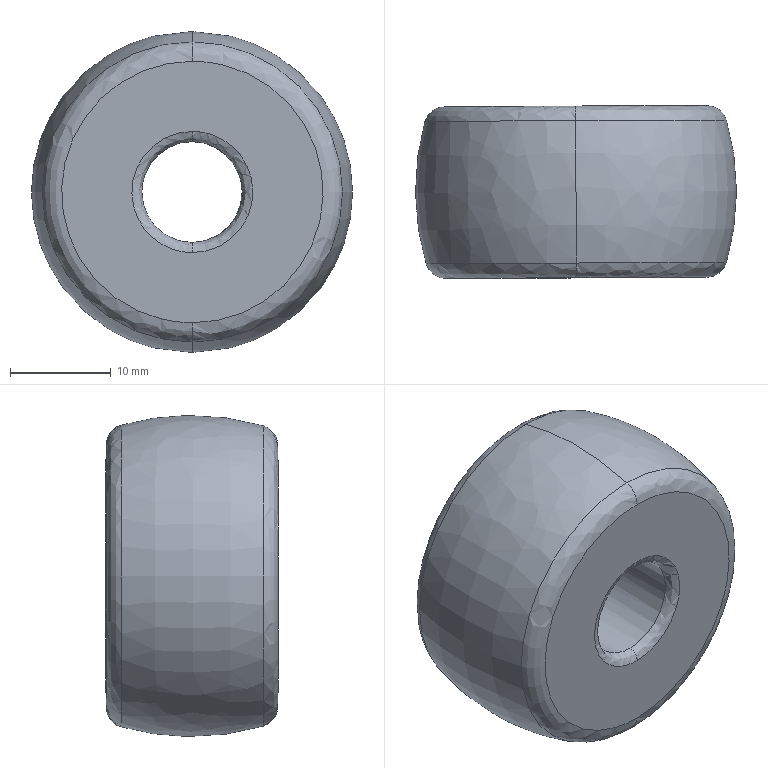Part | SolidWorks | features BaseBody 1 | 1 solid | 14 faces | box 31.826 x 17.113 x 31.826 mm | volume 11303 mm3 | spline 10 | cylinder 2 | plane 2 | commonest cylinder face diameters 10 x2
STEP:
#1=CARTESIAN_POINT('',(616.883,-156.463,-67.113));
#2=VERTEX_POINT('',#1);
#3=CARTESIAN_POINT('',(616.883,-156.463,-37.355));
#4=VERTEX_POINT('',#3);
#5=CARTESIAN_POINT('',(616.883,-156.463,-52.234));
#6=DIRECTION('',(0.004352,-1.,-0.000000003));
#7=DIRECTION('',(0.000000001,-0.000000003,1.));
#8=AXIS2_PLACEMENT_3D('',#5,#6,#7);
#9=CIRCLE('',#8,14.879);
#10=EDGE_CURVE('',#2,#4,#9,.T.);
#11=ORIENTED_EDGE('',*,*,#10,.F.);
#12=CARTESIAN_POINT('',(616.822,-142.349,-67.176));
#13=VERTEX_POINT('',#12);
#14=CARTESIAN_POINT('',(616.883,-156.463,-67.113));
#15=CARTESIAN_POINT('',(616.878,-155.365,-67.437));
#16=CARTESIAN_POINT('',(616.868,-153.033,-67.956));
#17=CARTESIAN_POINT('',(616.852,-149.411,-68.238));
#18=CARTESIAN_POINT('',(616.837,-145.786,-67.988));
#19=CARTESIAN_POINT('',(616.826,-143.45,-67.49));
#20=CARTESIAN_POINT('',(616.822,-142.349,-67.176));
#21=B_SPLINE_CURVE_WITH_KNOTS('',3,(#14,#15,#16,#17,#18,#19,#20),.UNSPECIFIED.,.F.,.F.,(4,1,1,1,4),(0.01923,0.25,0.5,0.75,0.9808),.UNSPECIFIED.);
#22=EDGE_CURVE('',#2,#13,#21,.T.);
#23=ORIENTED_EDGE('',*,*,#22,.T.);
#24=CARTESIAN_POINT('',(616.822,-142.349,-37.292));
#25=VERTEX_POINT('',#24);
#26=CARTESIAN_POINT('',(616.822,-142.349,-52.234));
#27=DIRECTION('',(-0.004352,1.,0.000000003));
#28=DIRECTION('',(0.000000001,-0.000000003,1.));
#29=AXIS2_PLACEMENT_3D('',#26,#27,#28);
#30=CIRCLE('',#29,14.942);
#31=EDGE_CURVE('',#25,#13,#30,.T.);
#32=ORIENTED_EDGE('',*,*,#31,.F.);
#33=CARTESIAN_POINT('',(616.883,-156.463,-37.355));
#34=CARTESIAN_POINT('',(616.878,-155.365,-37.031));
#35=CARTESIAN_POINT('',(616.868,-153.033,-36.513));
#36=CARTESIAN_POINT('',(616.852,-149.411,-36.23));
#37=CARTESIAN_POINT('',(616.837,-145.786,-36.48));
#38=CARTESIAN_POINT('',(616.826,-143.45,-36.979));
#39=CARTESIAN_POINT('',(616.822,-142.349,-37.292));
#40=B_SPLINE_CURVE_WITH_KNOTS('',3,(#33,#34,#35,#36,#37,#38,#39),.UNSPECIFIED.,.F.,.F.,(4,1,1,1,4),(0.01923,0.25,0.5,0.75,0.9808),.UNSPECIFIED.);
#41=EDGE_CURVE('',#4,#25,#40,.T.);
#42=ORIENTED_EDGE('',*,*,#41,.F.);
#43=EDGE_LOOP('',(#11,#23,#32,#42));
#44=FACE_OUTER_BOUND('',#43,.T.);
#45=CARTESIAN_POINT('',(616.883,-156.463,-37.355));
#46=CARTESIAN_POINT('',(646.641,-156.333,-37.355));
#47=CARTESIAN_POINT('',(646.641,-156.333,-67.113));
#48=CARTESIAN_POINT('',(616.883,-156.463,-67.113));
#49=CARTESIAN_POINT('',(616.878,-155.365,-37.031));
#50=CARTESIAN_POINT('',(647.284,-155.233,-37.031));
#51=CARTESIAN_POINT('',(647.284,-155.233,-67.437));
#52=CARTESIAN_POINT('',(616.878,-155.365,-67.437));
#53=CARTESIAN_POINT('',(616.868,-153.033,-36.513));
#54=CARTESIAN_POINT('',(648.311,-152.896,-36.513));
#55=CARTESIAN_POINT('',(648.311,-152.896,-67.956));
#56=CARTESIAN_POINT('',(616.868,-153.033,-67.956));
#57=CARTESIAN_POINT('',(616.852,-149.411,-36.23));
#58=CARTESIAN_POINT('',(648.86,-149.272,-36.23));
#59=CARTESIAN_POINT('',(648.86,-149.272,-68.238));
#60=CARTESIAN_POINT('',(616.852,-149.411,-68.238));
#61=CARTESIAN_POINT('',(616.837,-145.786,-36.48));
#62=CARTESIAN_POINT('',(648.344,-145.649,-36.48));
#63=CARTESIAN_POINT('',(648.344,-145.649,-67.988));
#64=CARTESIAN_POINT('',(616.837,-145.786,-67.988));
#65=CARTESIAN_POINT('',(616.826,-143.45,-36.979));
#66=CARTESIAN_POINT('',(647.337,-143.317,-36.979));
#67=CARTESIAN_POINT('',(647.337,-143.317,-67.49));
#68=CARTESIAN_POINT('',(616.826,-143.45,-67.49));
#69=CARTESIAN_POINT('',(616.822,-142.349,-37.292));
#70=CARTESIAN_POINT('',(646.705,-142.219,-37.292));
#71=CARTESIAN_POINT('',(646.705,-142.219,-67.176));
#72=CARTESIAN_POINT('',(616.822,-142.349,-67.176));
#73=(BOUNDED_SURFACE()B_SPLINE_SURFACE(3,3,((#45,#46,#47,#48),(#49,#50,#51,#52),(#53,#54,#55,#56),(#57,#58,#59,#60),(#61,#62,#63,#64),(#65,#66,#67,#68),(#69,#70,#71,#72)),.UNSPECIFIED.,.F.,.F.,.F.)B_SPLINE_SURFACE_WITH_KNOTS((4,1,1,1,4),(4,4),(0.01923,0.25,0.5,0.75,0.9808),(0.,1.),.UNSPECIFIED.)GEOMETRIC_REPRESENTATION_ITEM()RATIONAL_B_SPLINE_SURFACE(((1.,0.3333,0.3333,1.),(1.,0.3333,0.3333,1.),(1.,0.3333,0.3333,1.),(1.,0.3333,0.3333,1.),(1.,0.3333,0.3333,1.),(1.,0.3333,0.3333,1.),(1.,0.3333,0.3333,1.)))REPRESENTATION_ITEM('')SURFACE());
#74=ADVANCED_FACE('',(#44),#73,.F.);
#75=ORIENTED_EDGE('',*,*,#31,.T.);
#76=CARTESIAN_POINT('',(616.815,-140.898,-65.253));
#77=VERTEX_POINT('',#76);
#78=CARTESIAN_POINT('',(616.822,-142.349,-67.176));
#79=CARTESIAN_POINT('',(616.821,-142.15,-67.119));
#80=CARTESIAN_POINT('',(616.819,-141.754,-66.936));
#81=CARTESIAN_POINT('',(616.817,-141.271,-66.48));
#82=CARTESIAN_POINT('',(616.816,-140.965,-65.89));
#83=CARTESIAN_POINT('',(616.815,-140.898,-65.459));
#84=CARTESIAN_POINT('',(616.815,-140.898,-65.253));
#85=B_SPLINE_CURVE_WITH_KNOTS('',3,(#78,#79,#80,#81,#82,#83,#84),.UNSPECIFIED.,.F.,.F.,(4,1,1,1,4),(0.01923,0.25,0.5,0.75,0.9808),.UNSPECIFIED.);
#86=EDGE_CURVE('',#13,#77,#85,.T.);
#87=ORIENTED_EDGE('',*,*,#86,.T.);
#88=CARTESIAN_POINT('',(616.815,-140.898,-39.216));
#89=VERTEX_POINT('',#88);
#90=CARTESIAN_POINT('',(616.815,-140.898,-39.216));
#91=CARTESIAN_POINT('',(617.67,-140.894,-39.216));
#92=CARTESIAN_POINT('',(618.517,-140.89,-39.299));
#93=CARTESIAN_POINT('',(620.193,-140.883,-39.632));
#94=CARTESIAN_POINT('',(621.008,-140.879,-39.88));
#95=CARTESIAN_POINT('',(622.587,-140.872,-40.534));
#96=CARTESIAN_POINT('',(623.338,-140.869,-40.935));
#97=CARTESIAN_POINT('',(624.758,-140.863,-41.884));
#98=CARTESIAN_POINT('',(625.417,-140.86,-42.425));
#99=CARTESIAN_POINT('',(626.625,-140.855,-43.633));
#100=CARTESIAN_POINT('',(627.165,-140.853,-44.291));
#101=CARTESIAN_POINT('',(628.114,-140.848,-45.712));
#102=CARTESIAN_POINT('',(628.516,-140.847,-46.463));
#103=CARTESIAN_POINT('',(629.17,-140.844,-48.042));
#104=CARTESIAN_POINT('',(629.417,-140.843,-48.856));
#105=CARTESIAN_POINT('',(629.75,-140.841,-50.532));
#106=CARTESIAN_POINT('',(629.834,-140.841,-51.38));
#107=CARTESIAN_POINT('',(629.834,-140.841,-53.089));
#108=CARTESIAN_POINT('',(629.75,-140.841,-53.936));
#109=CARTESIAN_POINT('',(629.417,-140.843,-55.612));
#110=CARTESIAN_POINT('',(629.17,-140.844,-56.427));
#111=CARTESIAN_POINT('',(628.516,-140.847,-58.005));
#112=CARTESIAN_POINT('',(628.114,-140.848,-58.756));
#113=CARTESIAN_POINT('',(627.165,-140.853,-60.177));
#114=CARTESIAN_POINT('',(626.625,-140.855,-60.835));
#115=CARTESIAN_POINT('',(625.417,-140.86,-62.044));
#116=CARTESIAN_POINT('',(624.758,-140.863,-62.584));
#117=CARTESIAN_POINT('',(623.338,-140.869,-63.533));
#118=CARTESIAN_POINT('',(622.587,-140.872,-63.935));
#119=CARTESIAN_POINT('',(621.008,-140.879,-64.589));
#120=CARTESIAN_POINT('',(620.193,-140.883,-64.836));
#121=CARTESIAN_POINT('',(618.517,-140.89,-65.169));
#122=CARTESIAN_POINT('',(617.67,-140.894,-65.253));
#123=CARTESIAN_POINT('',(616.815,-140.898,-65.253));
#124=B_SPLINE_CURVE_WITH_KNOTS('',3,(#90,#91,#92,#93,#94,#95,#96,#97,#98,#99,#100,#101,#102,#103,#104,#105,#106,#107,#108,#109,#110,#111,#112,#113,#114,#115,#116,#117,#118,#119,#120,#121,#122,#123),.UNSPECIFIED.,.F.,.F.,(4,2,2,2,2,2,2,2,2,2,2,2,2,2,2,2,4),(0.,0.0625,0.125,0.1875,0.25,0.3125,0.375,0.4375,0.5,0.5625,0.625,0.6875,0.75,0.8125,0.875,0.9375,1.),.UNSPECIFIED.);
#125=EDGE_CURVE('',#89,#77,#124,.T.);
#126=ORIENTED_EDGE('',*,*,#125,.F.);
#127=CARTESIAN_POINT('',(616.822,-142.349,-37.292));
#128=CARTESIAN_POINT('',(616.821,-142.15,-37.349));
#129=CARTESIAN_POINT('',(616.819,-141.754,-37.532));
#130=CARTESIAN_POINT('',(616.817,-141.271,-37.988));
#131=CARTESIAN_POINT('',(616.816,-140.965,-38.578));
#132=CARTESIAN_POINT('',(616.815,-140.898,-39.009));
#133=CARTESIAN_POINT('',(616.815,-140.898,-39.216));
#134=B_SPLINE_CURVE_WITH_KNOTS('',3,(#127,#128,#129,#130,#131,#132,#133),.UNSPECIFIED.,.F.,.F.,(4,1,1,1,4),(0.01923,0.25,0.5,0.75,0.9808),.UNSPECIFIED.);
#135=EDGE_CURVE('',#25,#89,#134,.T.);
#136=ORIENTED_EDGE('',*,*,#135,.F.);
#137=EDGE_LOOP('',(#75,#87,#126,#136));
#138=FACE_OUTER_BOUND('',#137,.T.);
#139=CARTESIAN_POINT('',(616.822,-142.349,-37.292));
#140=CARTESIAN_POINT('',(646.705,-142.219,-37.292));
#141=CARTESIAN_POINT('',(646.705,-142.219,-67.176));
#142=CARTESIAN_POINT('',(616.822,-142.349,-67.176));
#143=CARTESIAN_POINT('',(616.821,-142.15,-37.349));
#144=CARTESIAN_POINT('',(646.591,-142.021,-37.349));
#145=CARTESIAN_POINT('',(646.591,-142.021,-67.119));
#146=CARTESIAN_POINT('',(616.821,-142.15,-67.119));
#147=CARTESIAN_POINT('',(616.819,-141.754,-37.532));
#148=CARTESIAN_POINT('',(646.223,-141.626,-37.532));
#149=CARTESIAN_POINT('',(646.223,-141.626,-66.936));
#150=CARTESIAN_POINT('',(616.819,-141.754,-66.936));
#151=CARTESIAN_POINT('',(616.817,-141.271,-37.988));
#152=CARTESIAN_POINT('',(645.309,-141.147,-37.988));
#153=CARTESIAN_POINT('',(645.309,-141.147,-66.48));
#154=CARTESIAN_POINT('',(616.817,-141.271,-66.48));
#155=CARTESIAN_POINT('',(616.816,-140.965,-38.578));
#156=CARTESIAN_POINT('',(644.128,-140.846,-38.578));
#157=CARTESIAN_POINT('',(644.128,-140.846,-65.89));
#158=CARTESIAN_POINT('',(616.816,-140.965,-65.89));
#159=CARTESIAN_POINT('',(616.815,-140.898,-39.009));
#160=CARTESIAN_POINT('',(643.266,-140.782,-39.009));
#161=CARTESIAN_POINT('',(643.266,-140.782,-65.459));
#162=CARTESIAN_POINT('',(616.815,-140.898,-65.459));
#163=CARTESIAN_POINT('',(616.815,-140.898,-39.216));
#164=CARTESIAN_POINT('',(642.852,-140.784,-39.216));
#165=CARTESIAN_POINT('',(642.852,-140.784,-65.253));
#166=CARTESIAN_POINT('',(616.815,-140.898,-65.253));
#167=(BOUNDED_SURFACE()B_SPLINE_SURFACE(3,3,((#139,#140,#141,#142),(#143,#144,#145,#146),(#147,#148,#149,#150),(#151,#152,#153,#154),(#155,#156,#157,#158),(#159,#160,#161,#162),(#163,#164,#165,#166)),.UNSPECIFIED.,.F.,.F.,.F.)B_SPLINE_SURFACE_WITH_KNOTS((4,1,1,1,4),(4,4),(0.01923,0.25,0.5,0.75,0.9808),(0.,1.),.UNSPECIFIED.)GEOMETRIC_REPRESENTATION_ITEM()RATIONAL_B_SPLINE_SURFACE(((1.,0.3333,0.3333,1.),(1.,0.3333,0.3333,1.),(1.,0.3333,0.3333,1.),(1.,0.3333,0.3333,1.),(1.,0.3333,0.3333,1.),(1.,0.3333,0.3333,1.),(1.,0.3333,0.3333,1.)))REPRESENTATION_ITEM('')SURFACE());
#168=ADVANCED_FACE('',(#138),#167,.F.);
#169=CARTESIAN_POINT('',(616.889,-157.897,-65.195));
#170=VERTEX_POINT('',#169);
#171=CARTESIAN_POINT('',(616.889,-157.897,-39.273));
#172=VERTEX_POINT('',#171);
#173=CARTESIAN_POINT('',(616.889,-157.897,-65.195));
#174=CARTESIAN_POINT('',(617.74,-157.894,-65.195));
#175=CARTESIAN_POINT('',(618.584,-157.89,-65.112));
#176=CARTESIAN_POINT('',(620.252,-157.883,-64.78));
#177=CARTESIAN_POINT('',(621.063,-157.879,-64.534));
#178=CARTESIAN_POINT('',(622.635,-157.872,-63.883));
#179=CARTESIAN_POINT('',(623.383,-157.869,-63.483));
#180=CARTESIAN_POINT('',(624.797,-157.863,-62.538));
#181=CARTESIAN_POINT('',(625.452,-157.86,-62.));
#182=CARTESIAN_POINT('',(626.656,-157.855,-60.797));
#183=CARTESIAN_POINT('',(627.193,-157.853,-60.142));
#184=CARTESIAN_POINT('',(628.138,-157.848,-58.728));
#185=CARTESIAN_POINT('',(628.538,-157.847,-57.98));
#186=CARTESIAN_POINT('',(629.189,-157.844,-56.408));
#187=CARTESIAN_POINT('',(629.435,-157.843,-55.597));
#188=CARTESIAN_POINT('',(629.767,-157.841,-53.928));
#189=CARTESIAN_POINT('',(629.85,-157.841,-53.085));
#190=CARTESIAN_POINT('',(629.85,-157.841,-51.383));
#191=CARTESIAN_POINT('',(629.767,-157.841,-50.54));
#192=CARTESIAN_POINT('',(629.435,-157.843,-48.871));
#193=CARTESIAN_POINT('',(629.189,-157.844,-48.06));
#194=CARTESIAN_POINT('',(628.538,-157.847,-46.488));
#195=CARTESIAN_POINT('',(628.138,-157.848,-45.741));
#196=CARTESIAN_POINT('',(627.193,-157.853,-44.326));
#197=CARTESIAN_POINT('',(626.655,-157.855,-43.671));
#198=CARTESIAN_POINT('',(625.453,-157.86,-42.468));
#199=CARTESIAN_POINT('',(624.797,-157.863,-41.93));
#200=CARTESIAN_POINT('',(623.383,-157.869,-40.985));
#201=CARTESIAN_POINT('',(622.635,-157.872,-40.585));
#202=CARTESIAN_POINT('',(621.063,-157.879,-39.934));
#203=CARTESIAN_POINT('',(620.252,-157.883,-39.688));
#204=CARTESIAN_POINT('',(618.583,-157.89,-39.356));
#205=CARTESIAN_POINT('',(617.741,-157.894,-39.273));
#206=CARTESIAN_POINT('',(616.889,-157.897,-39.273));
#207=B_SPLINE_CURVE_WITH_KNOTS('',3,(#173,#174,#175,#176,#177,#178,#179,#180,#181,#182,#183,#184,#185,#186,#187,#188,#189,#190,#191,#192,#193,#194,#195,#196,#197,#198,#199,#200,#201,#202,#203,#204,#205,#206),.UNSPECIFIED.,.F.,.F.,(4,2,2,2,2,2,2,2,2,2,2,2,2,2,2,2,4),(0.,0.0625,0.125,0.1875,0.25,0.3125,0.375,0.4375,0.5,0.5625,0.625,0.6875,0.75,0.8125,0.875,0.9375,1.),.UNSPECIFIED.);
#208=EDGE_CURVE('',#170,#172,#207,.T.);
#209=ORIENTED_EDGE('',*,*,#208,.F.);
#210=CARTESIAN_POINT('',(616.889,-157.897,-65.195));
#211=CARTESIAN_POINT('',(616.889,-157.897,-65.4));
#212=CARTESIAN_POINT('',(616.889,-157.831,-65.829));
#213=CARTESIAN_POINT('',(616.888,-157.529,-66.415));
#214=CARTESIAN_POINT('',(616.886,-157.052,-66.871));
#215=CARTESIAN_POINT('',(616.884,-156.66,-67.055));
#216=CARTESIAN_POINT('',(616.883,-156.463,-67.113));
#217=B_SPLINE_CURVE_WITH_KNOTS('',3,(#210,#211,#212,#213,#214,#215,#216),.UNSPECIFIED.,.F.,.F.,(4,1,1,1,4),(0.01923,0.25,0.5,0.75,0.9808),.UNSPECIFIED.);
#218=EDGE_CURVE('',#170,#2,#217,.T.);
#219=ORIENTED_EDGE('',*,*,#218,.T.);
#220=ORIENTED_EDGE('',*,*,#10,.T.);
#221=CARTESIAN_POINT('',(616.889,-157.897,-39.273));
#222=CARTESIAN_POINT('',(616.889,-157.897,-39.068));
#223=CARTESIAN_POINT('',(616.889,-157.831,-38.64));
#224=CARTESIAN_POINT('',(616.888,-157.529,-38.053));
#225=CARTESIAN_POINT('',(616.886,-157.052,-37.598));
#226=CARTESIAN_POINT('',(616.884,-156.66,-37.413));
#227=CARTESIAN_POINT('',(616.883,-156.463,-37.355));
#228=B_SPLINE_CURVE_WITH_KNOTS('',3,(#221,#222,#223,#224,#225,#226,#227),.UNSPECIFIED.,.F.,.F.,(4,1,1,1,4),(0.01923,0.25,0.5,0.75,0.9808),.UNSPECIFIED.);
#229=EDGE_CURVE('',#172,#4,#228,.T.);
#230=ORIENTED_EDGE('',*,*,#229,.F.);
#231=EDGE_LOOP('',(#209,#219,#220,#230));
#232=FACE_OUTER_BOUND('',#231,.T.);
#233=CARTESIAN_POINT('',(616.889,-157.897,-39.273));
#234=CARTESIAN_POINT('',(642.811,-157.785,-39.273));
#235=CARTESIAN_POINT('',(642.811,-157.785,-65.195));
#236=CARTESIAN_POINT('',(616.889,-157.897,-65.195));
#237=CARTESIAN_POINT('',(616.889,-157.897,-39.068));
#238=CARTESIAN_POINT('',(643.222,-157.783,-39.068));
#239=CARTESIAN_POINT('',(643.222,-157.783,-65.4));
#240=CARTESIAN_POINT('',(616.889,-157.897,-65.4));
#241=CARTESIAN_POINT('',(616.889,-157.831,-38.64));
#242=CARTESIAN_POINT('',(644.078,-157.713,-38.64));
#243=CARTESIAN_POINT('',(644.078,-157.713,-65.829));
#244=CARTESIAN_POINT('',(616.889,-157.831,-65.829));
#245=CARTESIAN_POINT('',(616.888,-157.529,-38.053));
#246=CARTESIAN_POINT('',(645.25,-157.406,-38.053));
#247=CARTESIAN_POINT('',(645.25,-157.406,-66.415));
#248=CARTESIAN_POINT('',(616.888,-157.529,-66.415));
#249=CARTESIAN_POINT('',(616.886,-157.052,-37.598));
#250=CARTESIAN_POINT('',(646.158,-156.924,-37.598));
#251=CARTESIAN_POINT('',(646.158,-156.924,-66.871));
#252=CARTESIAN_POINT('',(616.886,-157.052,-66.871));
#253=CARTESIAN_POINT('',(616.884,-156.66,-37.413));
#254=CARTESIAN_POINT('',(646.526,-156.531,-37.413));
#255=CARTESIAN_POINT('',(646.526,-156.531,-67.055));
#256=CARTESIAN_POINT('',(616.884,-156.66,-67.055));
#257=CARTESIAN_POINT('',(616.883,-156.463,-37.355));
#258=CARTESIAN_POINT('',(646.641,-156.333,-37.355));
#259=CARTESIAN_POINT('',(646.641,-156.333,-67.113));
#260=CARTESIAN_POINT('',(616.883,-156.463,-67.113));
#261=(BOUNDED_SURFACE()B_SPLINE_SURFACE(3,3,((#233,#234,#235,#236),(#237,#238,#239,#240),(#241,#242,#243,#244),(#245,#246,#247,#248),(#249,#250,#251,#252),(#253,#254,#255,#256),(#257,#258,#259,#260)),.UNSPECIFIED.,.F.,.F.,.F.)B_SPLINE_SURFACE_WITH_KNOTS((4,1,1,1,4),(4,4),(0.01923,0.25,0.5,0.75,0.9808),(0.,1.),.UNSPECIFIED.)GEOMETRIC_REPRESENTATION_ITEM()RATIONAL_B_SPLINE_SURFACE(((1.,0.3333,0.3333,1.),(1.,0.3333,0.3333,1.),(1.,0.3333,0.3333,1.),(1.,0.3333,0.3333,1.),(1.,0.3333,0.3333,1.),(1.,0.3333,0.3333,1.),(1.,0.3333,0.3333,1.)))REPRESENTATION_ITEM('')SURFACE());
#262=ADVANCED_FACE('',(#232),#261,.F.);
#263=CARTESIAN_POINT('',(616.815,-140.898,-58.234));
#264=VERTEX_POINT('',#263);
#265=CARTESIAN_POINT('',(616.815,-140.898,-46.234));
#266=VERTEX_POINT('',#265);
#267=CARTESIAN_POINT('',(616.815,-140.898,-58.234));
#268=CARTESIAN_POINT('',(617.603,-140.894,-58.234));
#269=CARTESIAN_POINT('',(618.384,-140.891,-58.079));
#270=CARTESIAN_POINT('',(619.839,-140.884,-57.476));
#271=CARTESIAN_POINT('',(620.501,-140.882,-57.033));
#272=CARTESIAN_POINT('',(621.615,-140.877,-55.92));
#273=CARTESIAN_POINT('',(622.057,-140.875,-55.257));
#274=CARTESIAN_POINT('',(622.66,-140.872,-53.803));
#275=CARTESIAN_POINT('',(622.815,-140.871,-53.021));
#276=CARTESIAN_POINT('',(622.815,-140.871,-51.447));
#277=CARTESIAN_POINT('',(622.66,-140.872,-50.665));
#278=CARTESIAN_POINT('',(622.057,-140.875,-49.211));
#279=CARTESIAN_POINT('',(621.615,-140.877,-48.548));
#280=CARTESIAN_POINT('',(620.501,-140.882,-47.435));
#281=CARTESIAN_POINT('',(619.839,-140.884,-46.992));
#282=CARTESIAN_POINT('',(618.748,-140.889,-46.54));
#283=CARTESIAN_POINT('',(618.372,-140.891,-46.426));
#284=CARTESIAN_POINT('',(617.6,-140.894,-46.273));
#285=CARTESIAN_POINT('',(617.21,-140.896,-46.234));
#286=CARTESIAN_POINT('',(616.815,-140.898,-46.234));
#287=B_SPLINE_CURVE_WITH_KNOTS('',3,(#267,#268,#269,#270,#271,#272,#273,#274,#275,#276,#277,#278,#279,#280,#281,#282,#283,#284,#285,#286),.UNSPECIFIED.,.F.,.F.,(4,2,2,2,2,2,2,2,2,4),(0.,0.125,0.25,0.375,0.5,0.625,0.75,0.875,0.9375,1.),.UNSPECIFIED.);
#288=EDGE_CURVE('',#264,#266,#287,.T.);
#289=ORIENTED_EDGE('',*,*,#288,.F.);
#290=CARTESIAN_POINT('',(616.82,-141.898,-57.234));
#291=VERTEX_POINT('',#290);
#292=CARTESIAN_POINT('',(616.815,-140.898,-58.234));
#293=CARTESIAN_POINT('',(616.815,-140.898,-58.11));
#294=CARTESIAN_POINT('',(616.816,-140.947,-57.849));
#295=CARTESIAN_POINT('',(616.817,-141.17,-57.506));
#296=CARTESIAN_POINT('',(616.818,-141.512,-57.283));
#297=CARTESIAN_POINT('',(616.819,-141.774,-57.234));
#298=CARTESIAN_POINT('',(616.82,-141.898,-57.234));
#299=B_SPLINE_CURVE_WITH_KNOTS('',3,(#292,#293,#294,#295,#296,#297,#298),.UNSPECIFIED.,.F.,.F.,(4,1,1,1,4),(0.02628,0.25,0.5,0.75,0.9737),.UNSPECIFIED.);
#300=EDGE_CURVE('',#264,#291,#299,.T.);
#301=ORIENTED_EDGE('',*,*,#300,.T.);
#302=CARTESIAN_POINT('',(621.82,-141.876,-52.234));
#303=VERTEX_POINT('',#302);
#304=CARTESIAN_POINT('',(621.82,-141.876,-52.234));
#305=CARTESIAN_POINT('',(621.82,-141.876,-52.889));
#306=CARTESIAN_POINT('',(621.69,-141.876,-53.543));
#307=CARTESIAN_POINT('',(621.189,-141.879,-54.752));
#308=CARTESIAN_POINT('',(620.818,-141.88,-55.307));
#309=CARTESIAN_POINT('',(619.892,-141.884,-56.232));
#310=CARTESIAN_POINT('',(619.338,-141.887,-56.603));
#311=CARTESIAN_POINT('',(618.128,-141.892,-57.104));
#312=CARTESIAN_POINT('',(617.474,-141.895,-57.234));
#313=CARTESIAN_POINT('',(616.82,-141.898,-57.234));
#314=B_SPLINE_CURVE_WITH_KNOTS('',3,(#304,#305,#306,#307,#308,#309,#310,#311,#312,#313),.UNSPECIFIED.,.F.,.F.,(4,2,2,2,4),(0.5,0.625,0.75,0.875,1.),.UNSPECIFIED.);
#315=EDGE_CURVE('',#303,#291,#314,.T.);
#316=ORIENTED_EDGE('',*,*,#315,.F.);
#317=CARTESIAN_POINT('',(616.82,-141.898,-47.234));
#318=VERTEX_POINT('',#317);
#319=CARTESIAN_POINT('',(616.82,-141.898,-47.234));
#320=CARTESIAN_POINT('',(617.474,-141.895,-47.234));
#321=CARTESIAN_POINT('',(618.128,-141.892,-47.364));
#322=CARTESIAN_POINT('',(619.338,-141.887,-47.865));
#323=CARTESIAN_POINT('',(619.892,-141.884,-48.236));
#324=CARTESIAN_POINT('',(620.818,-141.88,-49.161));
#325=CARTESIAN_POINT('',(621.189,-141.879,-49.716));
#326=CARTESIAN_POINT('',(621.69,-141.876,-50.925));
#327=CARTESIAN_POINT('',(621.82,-141.876,-51.58));
#328=CARTESIAN_POINT('',(621.82,-141.876,-52.234));
#329=B_SPLINE_CURVE_WITH_KNOTS('',3,(#319,#320,#321,#322,#323,#324,#325,#326,#327,#328),.UNSPECIFIED.,.F.,.F.,(4,2,2,2,4),(0.,0.125,0.25,0.375,0.5),.UNSPECIFIED.);
#330=EDGE_CURVE('',#318,#303,#329,.T.);
#331=ORIENTED_EDGE('',*,*,#330,.F.);
#332=CARTESIAN_POINT('',(616.815,-140.898,-46.234));
#333=CARTESIAN_POINT('',(616.815,-140.898,-46.358));
#334=CARTESIAN_POINT('',(616.816,-140.947,-46.62));
#335=CARTESIAN_POINT('',(616.817,-141.17,-46.962));
#336=CARTESIAN_POINT('',(616.818,-141.512,-47.185));
#337=CARTESIAN_POINT('',(616.819,-141.774,-47.234));
#338=CARTESIAN_POINT('',(616.82,-141.898,-47.234));
#339=B_SPLINE_CURVE_WITH_KNOTS('',3,(#332,#333,#334,#335,#336,#337,#338),.UNSPECIFIED.,.F.,.F.,(4,1,1,1,4),(0.02628,0.25,0.5,0.75,0.9737),.UNSPECIFIED.);
#340=EDGE_CURVE('',#266,#318,#339,.T.);
#341=ORIENTED_EDGE('',*,*,#340,.F.);
#342=EDGE_LOOP('',(#289,#301,#316,#331,#341));
#343=FACE_OUTER_BOUND('',#342,.T.);
#344=CARTESIAN_POINT('',(616.815,-140.898,-46.234));
#345=CARTESIAN_POINT('',(628.815,-140.845,-46.234));
#346=CARTESIAN_POINT('',(628.815,-140.845,-58.234));
#347=CARTESIAN_POINT('',(616.815,-140.898,-58.234));
#348=CARTESIAN_POINT('',(616.815,-140.898,-46.358));
#349=CARTESIAN_POINT('',(628.568,-140.846,-46.358));
#350=CARTESIAN_POINT('',(628.568,-140.846,-58.11));
#351=CARTESIAN_POINT('',(616.815,-140.898,-58.11));
#352=CARTESIAN_POINT('',(616.816,-140.947,-46.62));
#353=CARTESIAN_POINT('',(628.045,-140.898,-46.62));
#354=CARTESIAN_POINT('',(628.045,-140.898,-57.849));
#355=CARTESIAN_POINT('',(616.816,-140.947,-57.849));
#356=CARTESIAN_POINT('',(616.817,-141.17,-46.962));
#357=CARTESIAN_POINT('',(627.361,-141.124,-46.962));
#358=CARTESIAN_POINT('',(627.361,-141.124,-57.506));
#359=CARTESIAN_POINT('',(616.817,-141.17,-57.506));
#360=CARTESIAN_POINT('',(616.818,-141.512,-47.185));
#361=CARTESIAN_POINT('',(626.916,-141.468,-47.185));
#362=CARTESIAN_POINT('',(626.916,-141.468,-57.283));
#363=CARTESIAN_POINT('',(616.818,-141.512,-57.283));
#364=CARTESIAN_POINT('',(616.819,-141.774,-47.234));
#365=CARTESIAN_POINT('',(626.819,-141.73,-47.234));
#366=CARTESIAN_POINT('',(626.819,-141.73,-57.234));
#367=CARTESIAN_POINT('',(616.819,-141.774,-57.234));
#368=CARTESIAN_POINT('',(616.82,-141.898,-47.234));
#369=CARTESIAN_POINT('',(626.82,-141.854,-47.234));
#370=CARTESIAN_POINT('',(626.82,-141.854,-57.234));
#371=CARTESIAN_POINT('',(616.82,-141.898,-57.234));
#372=(BOUNDED_SURFACE()B_SPLINE_SURFACE(3,3,((#344,#345,#346,#347),(#348,#349,#350,#351),(#352,#353,#354,#355),(#356,#357,#358,#359),(#360,#361,#362,#363),(#364,#365,#366,#367),(#368,#369,#370,#371)),.UNSPECIFIED.,.F.,.F.,.T.)B_SPLINE_SURFACE_WITH_KNOTS((4,1,1,1,4),(4,4),(0.02628,0.25,0.5,0.75,0.9737),(0.,1.),.UNSPECIFIED.)GEOMETRIC_REPRESENTATION_ITEM()RATIONAL_B_SPLINE_SURFACE(((1.,0.3333,0.3333,1.),(1.,0.3333,0.3333,1.),(1.,0.3333,0.3333,1.),(1.,0.3333,0.3333,1.),(1.,0.3333,0.3333,1.),(1.,0.3333,0.3333,1.),(1.,0.3333,0.3333,1.)))REPRESENTATION_ITEM('')SURFACE());
#373=ADVANCED_FACE('',(#343),#372,.F.);
#374=CARTESIAN_POINT('',(616.885,-156.897,-57.234));
#375=VERTEX_POINT('',#374);
#376=CARTESIAN_POINT('',(621.885,-156.876,-52.234));
#377=VERTEX_POINT('',#376);
#378=CARTESIAN_POINT('',(616.885,-156.897,-57.234));
#379=CARTESIAN_POINT('',(617.54,-156.895,-57.234));
#380=CARTESIAN_POINT('',(618.194,-156.892,-57.104));
#381=CARTESIAN_POINT('',(619.403,-156.886,-56.603));
#382=CARTESIAN_POINT('',(619.958,-156.884,-56.232));
#383=CARTESIAN_POINT('',(620.883,-156.88,-55.307));
#384=CARTESIAN_POINT('',(621.254,-156.878,-54.752));
#385=CARTESIAN_POINT('',(621.755,-156.876,-53.543));
#386=CARTESIAN_POINT('',(621.885,-156.876,-52.889));
#387=CARTESIAN_POINT('',(621.885,-156.876,-52.234));
#388=B_SPLINE_CURVE_WITH_KNOTS('',3,(#378,#379,#380,#381,#382,#383,#384,#385,#386,#387),.UNSPECIFIED.,.F.,.F.,(4,2,2,2,4),(0.,0.125,0.25,0.375,0.5),.UNSPECIFIED.);
#389=EDGE_CURVE('',#375,#377,#388,.T.);
#390=ORIENTED_EDGE('',*,*,#389,.F.);
#391=CARTESIAN_POINT('',(616.889,-157.897,-58.234));
#392=VERTEX_POINT('',#391);
#393=CARTESIAN_POINT('',(616.885,-156.897,-57.234));
#394=CARTESIAN_POINT('',(616.886,-157.021,-57.234));
#395=CARTESIAN_POINT('',(616.887,-157.283,-57.283));
#396=CARTESIAN_POINT('',(616.888,-157.625,-57.506));
#397=CARTESIAN_POINT('',(616.889,-157.848,-57.849));
#398=CARTESIAN_POINT('',(616.889,-157.897,-58.11));
#399=CARTESIAN_POINT('',(616.889,-157.897,-58.234));
#400=B_SPLINE_CURVE_WITH_KNOTS('',3,(#393,#394,#395,#396,#397,#398,#399),.UNSPECIFIED.,.F.,.F.,(4,1,1,1,4),(0.02628,0.25,0.5,0.75,0.9737),.UNSPECIFIED.);
#401=EDGE_CURVE('',#375,#392,#400,.T.);
#402=ORIENTED_EDGE('',*,*,#401,.T.);
#403=CARTESIAN_POINT('',(616.889,-157.897,-46.234));
#404=VERTEX_POINT('',#403);
#405=CARTESIAN_POINT('',(616.889,-157.897,-58.234));
#406=CARTESIAN_POINT('',(628.889,-157.845,-58.234));
#407=CARTESIAN_POINT('',(628.889,-157.845,-46.234));
#408=CARTESIAN_POINT('',(616.889,-157.897,-46.234));
#409=(BOUNDED_CURVE()B_SPLINE_CURVE(3,(#405,#406,#407,#408),.UNSPECIFIED.,.F.,.F.)B_SPLINE_CURVE_WITH_KNOTS((4,4),(0.,1.),.UNSPECIFIED.)CURVE()GEOMETRIC_REPRESENTATION_ITEM()RATIONAL_B_SPLINE_CURVE((1.,0.3333,0.3333,1.))REPRESENTATION_ITEM(''));
#410=EDGE_CURVE('',#392,#404,#409,.T.);
#411=ORIENTED_EDGE('',*,*,#410,.T.);
#412=CARTESIAN_POINT('',(616.885,-156.897,-47.234));
#413=VERTEX_POINT('',#412);
#414=CARTESIAN_POINT('',(616.885,-156.897,-47.234));
#415=CARTESIAN_POINT('',(616.886,-157.021,-47.234));
#416=CARTESIAN_POINT('',(616.887,-157.283,-47.185));
#417=CARTESIAN_POINT('',(616.888,-157.625,-46.962));
#418=CARTESIAN_POINT('',(616.889,-157.848,-46.62));
#419=CARTESIAN_POINT('',(616.889,-157.897,-46.358));
#420=CARTESIAN_POINT('',(616.889,-157.897,-46.234));
#421=B_SPLINE_CURVE_WITH_KNOTS('',3,(#414,#415,#416,#417,#418,#419,#420),.UNSPECIFIED.,.F.,.F.,(4,1,1,1,4),(0.02628,0.25,0.5,0.75,0.9737),.UNSPECIFIED.);
#422=EDGE_CURVE('',#413,#404,#421,.T.);
#423=ORIENTED_EDGE('',*,*,#422,.F.);
#424=CARTESIAN_POINT('',(621.885,-156.876,-52.234));
#425=CARTESIAN_POINT('',(621.885,-156.876,-51.58));
#426=CARTESIAN_POINT('',(621.755,-156.876,-50.925));
#427=CARTESIAN_POINT('',(621.254,-156.878,-49.716));
#428=CARTESIAN_POINT('',(620.883,-156.88,-49.161));
#429=CARTESIAN_POINT('',(619.958,-156.884,-48.236));
#430=CARTESIAN_POINT('',(619.403,-156.886,-47.865));
#431=CARTESIAN_POINT('',(618.194,-156.892,-47.364));
#432=CARTESIAN_POINT('',(617.54,-156.895,-47.234));
#433=CARTESIAN_POINT('',(616.885,-156.897,-47.234));
#434=B_SPLINE_CURVE_WITH_KNOTS('',3,(#424,#425,#426,#427,#428,#429,#430,#431,#432,#433),.UNSPECIFIED.,.F.,.F.,(4,2,2,2,4),(0.5,0.625,0.75,0.875,1.),.UNSPECIFIED.);
#435=EDGE_CURVE('',#377,#413,#434,.T.);
#436=ORIENTED_EDGE('',*,*,#435,.F.);
#437=EDGE_LOOP('',(#390,#402,#411,#423,#436));
#438=FACE_OUTER_BOUND('',#437,.T.);
#439=CARTESIAN_POINT('',(616.885,-156.897,-47.234));
#440=CARTESIAN_POINT('',(626.885,-156.854,-47.234));
#441=CARTESIAN_POINT('',(626.885,-156.854,-57.234));
#442=CARTESIAN_POINT('',(616.885,-156.897,-57.234));
#443=CARTESIAN_POINT('',(616.886,-157.021,-47.234));
#444=CARTESIAN_POINT('',(626.886,-156.978,-47.234));
#445=CARTESIAN_POINT('',(626.886,-156.978,-57.234));
#446=CARTESIAN_POINT('',(616.886,-157.021,-57.234));
#447=CARTESIAN_POINT('',(616.887,-157.283,-47.185));
#448=CARTESIAN_POINT('',(626.985,-157.239,-47.185));
#449=CARTESIAN_POINT('',(626.985,-157.239,-57.283));
#450=CARTESIAN_POINT('',(616.887,-157.283,-57.283));
#451=CARTESIAN_POINT('',(616.888,-157.625,-46.962));
#452=CARTESIAN_POINT('',(627.433,-157.579,-46.962));
#453=CARTESIAN_POINT('',(627.433,-157.579,-57.506));
#454=CARTESIAN_POINT('',(616.888,-157.625,-57.506));
#455=CARTESIAN_POINT('',(616.889,-157.848,-46.62));
#456=CARTESIAN_POINT('',(628.118,-157.799,-46.62));
#457=CARTESIAN_POINT('',(628.118,-157.799,-57.849));
#458=CARTESIAN_POINT('',(616.889,-157.848,-57.849));
#459=CARTESIAN_POINT('',(616.889,-157.897,-46.358));
#460=CARTESIAN_POINT('',(628.642,-157.846,-46.358));
#461=CARTESIAN_POINT('',(628.642,-157.846,-58.11));
#462=CARTESIAN_POINT('',(616.889,-157.897,-58.11));
#463=CARTESIAN_POINT('',(616.889,-157.897,-46.234));
#464=CARTESIAN_POINT('',(628.889,-157.845,-46.234));
#465=CARTESIAN_POINT('',(628.889,-157.845,-58.234));
#466=CARTESIAN_POINT('',(616.889,-157.897,-58.234));
#467=(BOUNDED_SURFACE()B_SPLINE_SURFACE(3,3,((#439,#440,#441,#442),(#443,#444,#445,#446),(#447,#448,#449,#450),(#451,#452,#453,#454),(#455,#456,#457,#458),(#459,#460,#461,#462),(#463,#464,#465,#466)),.UNSPECIFIED.,.F.,.F.,.F.)B_SPLINE_SURFACE_WITH_KNOTS((4,1,1,1,4),(4,4),(0.02628,0.25,0.5,0.75,0.9737),(0.,1.),.UNSPECIFIED.)GEOMETRIC_REPRESENTATION_ITEM()RATIONAL_B_SPLINE_SURFACE(((1.,0.3333,0.3333,1.),(1.,0.3333,0.3333,1.),(1.,0.3333,0.3333,1.),(1.,0.3333,0.3333,1.),(1.,0.3333,0.3333,1.),(1.,0.3333,0.3333,1.),(1.,0.3333,0.3333,1.)))REPRESENTATION_ITEM('')SURFACE());
#468=ADVANCED_FACE('',(#438),#467,.F.);
#469=ORIENTED_EDGE('',*,*,#389,.T.);
#470=CARTESIAN_POINT('',(621.885,-156.876,-52.234));
#471=DIRECTION('',(-0.004352,1.,0.000000003));
#472=VECTOR('',#471,1000.);
#473=LINE('',#470,#472);
#474=EDGE_CURVE('',#377,#303,#473,.T.);
#475=ORIENTED_EDGE('',*,*,#474,.T.);
#476=ORIENTED_EDGE('',*,*,#315,.T.);
#477=CARTESIAN_POINT('',(611.82,-141.919,-52.234));
#478=VERTEX_POINT('',#477);
#479=CARTESIAN_POINT('',(616.82,-141.898,-57.234));
#480=CARTESIAN_POINT('',(616.165,-141.9,-57.234));
#481=CARTESIAN_POINT('',(615.511,-141.903,-57.104));
#482=CARTESIAN_POINT('',(614.302,-141.909,-56.603));
#483=CARTESIAN_POINT('',(613.747,-141.911,-56.232));
#484=CARTESIAN_POINT('',(612.821,-141.915,-55.307));
#485=CARTESIAN_POINT('',(612.451,-141.917,-54.752));
#486=CARTESIAN_POINT('',(611.95,-141.919,-53.543));
#487=CARTESIAN_POINT('',(611.82,-141.919,-52.889));
#488=CARTESIAN_POINT('',(611.82,-141.919,-52.234));
#489=B_SPLINE_CURVE_WITH_KNOTS('',3,(#479,#480,#481,#482,#483,#484,#485,#486,#487,#488),.UNSPECIFIED.,.F.,.F.,(4,2,2,2,4),(0.,0.125,0.25,0.375,0.5),.UNSPECIFIED.);
#490=EDGE_CURVE('',#291,#478,#489,.T.);
#491=ORIENTED_EDGE('',*,*,#490,.T.);
#492=CARTESIAN_POINT('',(611.885,-156.919,-52.234));
#493=VERTEX_POINT('',#492);
#494=CARTESIAN_POINT('',(611.885,-156.919,-52.234));
#495=DIRECTION('',(-0.004352,1.,0.000000003));
#496=VECTOR('',#495,1000.);
#497=LINE('',#494,#496);
#498=EDGE_CURVE('',#493,#478,#497,.T.);
#499=ORIENTED_EDGE('',*,*,#498,.F.);
#500=CARTESIAN_POINT('',(611.885,-156.919,-52.234));
#501=CARTESIAN_POINT('',(611.885,-156.919,-52.889));
#502=CARTESIAN_POINT('',(612.015,-156.919,-53.543));
#503=CARTESIAN_POINT('',(612.516,-156.916,-54.752));
#504=CARTESIAN_POINT('',(612.887,-156.915,-55.307));
#505=CARTESIAN_POINT('',(613.812,-156.911,-56.232));
#506=CARTESIAN_POINT('',(614.367,-156.908,-56.603));
#507=CARTESIAN_POINT('',(615.576,-156.903,-57.104));
#508=CARTESIAN_POINT('',(616.231,-156.9,-57.234));
#509=CARTESIAN_POINT('',(616.885,-156.897,-57.234));
#510=B_SPLINE_CURVE_WITH_KNOTS('',3,(#500,#501,#502,#503,#504,#505,#506,#507,#508,#509),.UNSPECIFIED.,.F.,.F.,(4,2,2,2,4),(0.5,0.625,0.75,0.875,1.),.UNSPECIFIED.);
#511=EDGE_CURVE('',#493,#375,#510,.T.);
#512=ORIENTED_EDGE('',*,*,#511,.T.);
#513=EDGE_LOOP('',(#469,#475,#476,#491,#499,#512));
#514=FACE_OUTER_BOUND('',#513,.T.);
#515=CARTESIAN_POINT('',(616.885,-156.897,-52.234));
#516=DIRECTION('',(-0.004352,1.,0.000000003));
#517=DIRECTION('',(-1.,-0.004352,0.));
#518=AXIS2_PLACEMENT_3D('',#515,#516,#517);
#519=CYLINDRICAL_SURFACE('',#518,5.);
#520=ADVANCED_FACE('',(#514),#519,.F.);
#521=ORIENTED_EDGE('',*,*,#22,.F.);
#522=CARTESIAN_POINT('',(616.883,-156.463,-52.234));
#523=DIRECTION('',(0.004352,-1.,-0.000000003));
#524=DIRECTION('',(0.000000001,-0.000000003,1.));
#525=AXIS2_PLACEMENT_3D('',#522,#523,#524);
#526=CIRCLE('',#525,14.879);
#527=EDGE_CURVE('',#4,#2,#526,.T.);
#528=ORIENTED_EDGE('',*,*,#527,.F.);
#529=ORIENTED_EDGE('',*,*,#41,.T.);
#530=CARTESIAN_POINT('',(616.822,-142.349,-52.234));
#531=DIRECTION('',(-0.004352,1.,0.000000003));
#532=DIRECTION('',(0.000000001,-0.000000003,1.));
#533=AXIS2_PLACEMENT_3D('',#530,#531,#532);
#534=CIRCLE('',#533,14.942);
#535=EDGE_CURVE('',#13,#25,#534,.T.);
#536=ORIENTED_EDGE('',*,*,#535,.F.);
#537=EDGE_LOOP('',(#521,#528,#529,#536));
#538=FACE_OUTER_BOUND('',#537,.T.);
#539=CARTESIAN_POINT('',(616.883,-156.463,-67.113));
#540=CARTESIAN_POINT('',(587.125,-156.592,-67.113));
#541=CARTESIAN_POINT('',(587.125,-156.592,-37.355));
#542=CARTESIAN_POINT('',(616.883,-156.463,-37.355));
#543=CARTESIAN_POINT('',(616.878,-155.365,-67.437));
#544=CARTESIAN_POINT('',(586.473,-155.498,-67.437));
#545=CARTESIAN_POINT('',(586.473,-155.498,-37.031));
#546=CARTESIAN_POINT('',(616.878,-155.365,-37.031));
#547=CARTESIAN_POINT('',(616.868,-153.033,-67.956));
#548=CARTESIAN_POINT('',(585.425,-153.17,-67.956));
#549=CARTESIAN_POINT('',(585.425,-153.17,-36.513));
#550=CARTESIAN_POINT('',(616.868,-153.033,-36.513));
#551=CARTESIAN_POINT('',(616.852,-149.411,-68.238));
#552=CARTESIAN_POINT('',(584.845,-149.55,-68.238));
#553=CARTESIAN_POINT('',(584.845,-149.55,-36.23));
#554=CARTESIAN_POINT('',(616.852,-149.411,-36.23));
#555=CARTESIAN_POINT('',(616.837,-145.786,-67.988));
#556=CARTESIAN_POINT('',(585.33,-145.923,-67.988));
#557=CARTESIAN_POINT('',(585.33,-145.923,-36.48));
#558=CARTESIAN_POINT('',(616.837,-145.786,-36.48));
#559=CARTESIAN_POINT('',(616.826,-143.45,-67.49));
#560=CARTESIAN_POINT('',(586.316,-143.582,-67.49));
#561=CARTESIAN_POINT('',(586.316,-143.582,-36.979));
#562=CARTESIAN_POINT('',(616.826,-143.45,-36.979));
#563=CARTESIAN_POINT('',(616.822,-142.349,-67.176));
#564=CARTESIAN_POINT('',(586.938,-142.479,-67.176));
#565=CARTESIAN_POINT('',(586.938,-142.479,-37.292));
#566=CARTESIAN_POINT('',(616.822,-142.349,-37.292));
#567=(BOUNDED_SURFACE()B_SPLINE_SURFACE(3,3,((#539,#540,#541,#542),(#543,#544,#545,#546),(#547,#548,#549,#550),(#551,#552,#553,#554),(#555,#556,#557,#558),(#559,#560,#561,#562),(#563,#564,#565,#566)),.UNSPECIFIED.,.F.,.F.,.F.)B_SPLINE_SURFACE_WITH_KNOTS((4,1,1,1,4),(4,4),(0.01923,0.25,0.5,0.75,0.9808),(0.,1.),.UNSPECIFIED.)GEOMETRIC_REPRESENTATION_ITEM()RATIONAL_B_SPLINE_SURFACE(((1.,0.3333,0.3333,1.),(1.,0.3333,0.3333,1.),(1.,0.3333,0.3333,1.),(1.,0.3333,0.3333,1.),(1.,0.3333,0.3333,1.),(1.,0.3333,0.3333,1.),(1.,0.3333,0.3333,1.)))REPRESENTATION_ITEM('')SURFACE());
#568=ADVANCED_FACE('',(#538),#567,.F.);
#569=ORIENTED_EDGE('',*,*,#86,.F.);
#570=ORIENTED_EDGE('',*,*,#535,.T.);
#571=ORIENTED_EDGE('',*,*,#135,.T.);
#572=CARTESIAN_POINT('',(616.815,-140.898,-65.253));
#573=CARTESIAN_POINT('',(615.961,-140.901,-65.253));
#574=CARTESIAN_POINT('',(615.114,-140.905,-65.169));
#575=CARTESIAN_POINT('',(613.438,-140.912,-64.836));
#576=CARTESIAN_POINT('',(612.623,-140.916,-64.589));
#577=CARTESIAN_POINT('',(611.044,-140.923,-63.935));
#578=CARTESIAN_POINT('',(610.293,-140.926,-63.533));
#579=CARTESIAN_POINT('',(608.872,-140.932,-62.584));
#580=CARTESIAN_POINT('',(608.214,-140.935,-62.044));
#581=CARTESIAN_POINT('',(607.006,-140.94,-60.835));
#582=CARTESIAN_POINT('',(606.466,-140.943,-60.177));
#583=CARTESIAN_POINT('',(605.516,-140.947,-58.756));
#584=CARTESIAN_POINT('',(605.115,-140.948,-58.005));
#585=CARTESIAN_POINT('',(604.461,-140.951,-56.427));
#586=CARTESIAN_POINT('',(604.214,-140.952,-55.612));
#587=CARTESIAN_POINT('',(603.88,-140.954,-53.936));
#588=CARTESIAN_POINT('',(603.797,-140.954,-53.089));
#589=CARTESIAN_POINT('',(603.797,-140.954,-51.38));
#590=CARTESIAN_POINT('',(603.881,-140.954,-50.532));
#591=CARTESIAN_POINT('',(604.214,-140.952,-48.856));
#592=CARTESIAN_POINT('',(604.461,-140.951,-48.042));
#593=CARTESIAN_POINT('',(605.115,-140.948,-46.463));
#594=CARTESIAN_POINT('',(605.516,-140.947,-45.712));
#595=CARTESIAN_POINT('',(606.466,-140.943,-44.291));
#596=CARTESIAN_POINT('',(607.006,-140.94,-43.633));
#597=CARTESIAN_POINT('',(608.214,-140.935,-42.424));
#598=CARTESIAN_POINT('',(608.872,-140.932,-41.884));
#599=CARTESIAN_POINT('',(610.293,-140.926,-40.935));
#600=CARTESIAN_POINT('',(611.044,-140.923,-40.534));
#601=CARTESIAN_POINT('',(612.623,-140.916,-39.88));
#602=CARTESIAN_POINT('',(613.437,-140.912,-39.633));
#603=CARTESIAN_POINT('',(615.114,-140.905,-39.299));
#604=CARTESIAN_POINT('',(615.96,-140.901,-39.216));
#605=CARTESIAN_POINT('',(616.815,-140.898,-39.216));
#606=B_SPLINE_CURVE_WITH_KNOTS('',3,(#572,#573,#574,#575,#576,#577,#578,#579,#580,#581,#582,#583,#584,#585,#586,#587,#588,#589,#590,#591,#592,#593,#594,#595,#596,#597,#598,#599,#600,#601,#602,#603,#604,#605),.UNSPECIFIED.,.F.,.F.,(4,2,2,2,2,2,2,2,2,2,2,2,2,2,2,2,4),(0.,0.0625,0.125,0.1875,0.25,0.3125,0.375,0.4375,0.5,0.5625,0.625,0.6875,0.75,0.8125,0.875,0.9375,1.),.UNSPECIFIED.);
#607=EDGE_CURVE('',#77,#89,#606,.T.);
#608=ORIENTED_EDGE('',*,*,#607,.F.);
#609=EDGE_LOOP('',(#569,#570,#571,#608));
#610=FACE_OUTER_BOUND('',#609,.T.);
#611=CARTESIAN_POINT('',(616.822,-142.349,-67.176));
#612=CARTESIAN_POINT('',(586.938,-142.479,-67.176));
#613=CARTESIAN_POINT('',(586.938,-142.479,-37.292));
#614=CARTESIAN_POINT('',(616.822,-142.349,-37.292));
#615=CARTESIAN_POINT('',(616.821,-142.15,-67.119));
#616=CARTESIAN_POINT('',(587.051,-142.28,-67.119));
#617=CARTESIAN_POINT('',(587.051,-142.28,-37.349));
#618=CARTESIAN_POINT('',(616.821,-142.15,-37.349));
#619=CARTESIAN_POINT('',(616.819,-141.754,-66.936));
#620=CARTESIAN_POINT('',(587.415,-141.882,-66.936));
#621=CARTESIAN_POINT('',(587.415,-141.882,-37.532));
#622=CARTESIAN_POINT('',(616.819,-141.754,-37.532));
#623=CARTESIAN_POINT('',(616.817,-141.271,-66.48));
#624=CARTESIAN_POINT('',(588.325,-141.395,-66.48));
#625=CARTESIAN_POINT('',(588.325,-141.395,-37.988));
#626=CARTESIAN_POINT('',(616.817,-141.271,-37.988));
#627=CARTESIAN_POINT('',(616.816,-140.965,-65.89));
#628=CARTESIAN_POINT('',(589.503,-141.084,-65.89));
#629=CARTESIAN_POINT('',(589.503,-141.084,-38.578));
#630=CARTESIAN_POINT('',(616.816,-140.965,-38.578));
#631=CARTESIAN_POINT('',(616.815,-140.898,-65.459));
#632=CARTESIAN_POINT('',(590.365,-141.013,-65.459));
#633=CARTESIAN_POINT('',(590.365,-141.013,-39.009));
#634=CARTESIAN_POINT('',(616.815,-140.898,-39.009));
#635=CARTESIAN_POINT('',(616.815,-140.898,-65.253));
#636=CARTESIAN_POINT('',(590.779,-141.011,-65.253));
#637=CARTESIAN_POINT('',(590.779,-141.011,-39.216));
#638=CARTESIAN_POINT('',(616.815,-140.898,-39.216));
#639=(BOUNDED_SURFACE()B_SPLINE_SURFACE(3,3,((#611,#612,#613,#614),(#615,#616,#617,#618),(#619,#620,#621,#622),(#623,#624,#625,#626),(#627,#628,#629,#630),(#631,#632,#633,#634),(#635,#636,#637,#638)),.UNSPECIFIED.,.F.,.F.,.F.)B_SPLINE_SURFACE_WITH_KNOTS((4,1,1,1,4),(4,4),(0.01923,0.25,0.5,0.75,0.9808),(0.,1.),.UNSPECIFIED.)GEOMETRIC_REPRESENTATION_ITEM()RATIONAL_B_SPLINE_SURFACE(((1.,0.3333,0.3333,1.),(1.,0.3333,0.3333,1.),(1.,0.3333,0.3333,1.),(1.,0.3333,0.3333,1.),(1.,0.3333,0.3333,1.),(1.,0.3333,0.3333,1.),(1.,0.3333,0.3333,1.)))REPRESENTATION_ITEM('')SURFACE());
#640=ADVANCED_FACE('',(#610),#639,.F.);
#641=ORIENTED_EDGE('',*,*,#218,.F.);
#642=CARTESIAN_POINT('',(616.889,-157.897,-39.273));
#643=CARTESIAN_POINT('',(616.039,-157.901,-39.273));
#644=CARTESIAN_POINT('',(615.195,-157.905,-39.356));
#645=CARTESIAN_POINT('',(613.527,-157.912,-39.688));
#646=CARTESIAN_POINT('',(612.715,-157.916,-39.934));
#647=CARTESIAN_POINT('',(611.144,-157.922,-40.585));
#648=CARTESIAN_POINT('',(610.396,-157.926,-40.985));
#649=CARTESIAN_POINT('',(608.981,-157.932,-41.93));
#650=CARTESIAN_POINT('',(608.326,-157.935,-42.468));
#651=CARTESIAN_POINT('',(607.123,-157.94,-43.671));
#652=CARTESIAN_POINT('',(606.586,-157.942,-44.326));
#653=CARTESIAN_POINT('',(605.64,-157.946,-45.741));
#654=CARTESIAN_POINT('',(605.241,-157.948,-46.488));
#655=CARTESIAN_POINT('',(604.59,-157.951,-48.06));
#656=CARTESIAN_POINT('',(604.344,-157.952,-48.871));
#657=CARTESIAN_POINT('',(604.012,-157.953,-50.54));
#658=CARTESIAN_POINT('',(603.929,-157.954,-51.383));
#659=CARTESIAN_POINT('',(603.929,-157.954,-53.085));
#660=CARTESIAN_POINT('',(604.012,-157.953,-53.928));
#661=CARTESIAN_POINT('',(604.344,-157.952,-55.597));
#662=CARTESIAN_POINT('',(604.59,-157.951,-56.408));
#663=CARTESIAN_POINT('',(605.241,-157.948,-57.98));
#664=CARTESIAN_POINT('',(605.64,-157.946,-58.727));
#665=CARTESIAN_POINT('',(606.585,-157.942,-60.142));
#666=CARTESIAN_POINT('',(607.123,-157.94,-60.797));
#667=CARTESIAN_POINT('',(608.326,-157.935,-62.));
#668=CARTESIAN_POINT('',(608.981,-157.932,-62.538));
#669=CARTESIAN_POINT('',(610.396,-157.926,-63.483));
#670=CARTESIAN_POINT('',(611.144,-157.922,-63.883));
#671=CARTESIAN_POINT('',(612.715,-157.916,-64.534));
#672=CARTESIAN_POINT('',(613.526,-157.912,-64.78));
#673=CARTESIAN_POINT('',(615.195,-157.905,-65.112));
#674=CARTESIAN_POINT('',(616.038,-157.901,-65.195));
#675=CARTESIAN_POINT('',(616.889,-157.897,-65.195));
#676=B_SPLINE_CURVE_WITH_KNOTS('',3,(#642,#643,#644,#645,#646,#647,#648,#649,#650,#651,#652,#653,#654,#655,#656,#657,#658,#659,#660,#661,#662,#663,#664,#665,#666,#667,#668,#669,#670,#671,#672,#673,#674,#675),.UNSPECIFIED.,.F.,.F.,(4,2,2,2,2,2,2,2,2,2,2,2,2,2,2,2,4),(0.,0.0625,0.125,0.1875,0.25,0.3125,0.375,0.4375,0.5,0.5625,0.625,0.6875,0.75,0.8125,0.875,0.9375,1.),.UNSPECIFIED.);
#677=EDGE_CURVE('',#172,#170,#676,.T.);
#678=ORIENTED_EDGE('',*,*,#677,.F.);
#679=ORIENTED_EDGE('',*,*,#229,.T.);
#680=ORIENTED_EDGE('',*,*,#527,.T.);
#681=EDGE_LOOP('',(#641,#678,#679,#680));
#682=FACE_OUTER_BOUND('',#681,.T.);
#683=CARTESIAN_POINT('',(616.889,-157.897,-65.195));
#684=CARTESIAN_POINT('',(590.968,-158.01,-65.195));
#685=CARTESIAN_POINT('',(590.968,-158.01,-39.273));
#686=CARTESIAN_POINT('',(616.889,-157.897,-39.273));
#687=CARTESIAN_POINT('',(616.889,-157.897,-65.4));
#688=CARTESIAN_POINT('',(590.557,-158.012,-65.4));
#689=CARTESIAN_POINT('',(590.557,-158.012,-39.068));
#690=CARTESIAN_POINT('',(616.889,-157.897,-39.068));
#691=CARTESIAN_POINT('',(616.889,-157.831,-65.829));
#692=CARTESIAN_POINT('',(589.701,-157.949,-65.829));
#693=CARTESIAN_POINT('',(589.701,-157.949,-38.64));
#694=CARTESIAN_POINT('',(616.889,-157.831,-38.64));
#695=CARTESIAN_POINT('',(616.888,-157.529,-66.415));
#696=CARTESIAN_POINT('',(588.526,-157.653,-66.415));
#697=CARTESIAN_POINT('',(588.526,-157.653,-38.053));
#698=CARTESIAN_POINT('',(616.888,-157.529,-38.053));
#699=CARTESIAN_POINT('',(616.886,-157.052,-66.871));
#700=CARTESIAN_POINT('',(587.613,-157.179,-66.871));
#701=CARTESIAN_POINT('',(587.613,-157.179,-37.598));
#702=CARTESIAN_POINT('',(616.886,-157.052,-37.598));
#703=CARTESIAN_POINT('',(616.884,-156.66,-67.055));
#704=CARTESIAN_POINT('',(587.242,-156.789,-67.055));
#705=CARTESIAN_POINT('',(587.242,-156.789,-37.413));
#706=CARTESIAN_POINT('',(616.884,-156.66,-37.413));
#707=CARTESIAN_POINT('',(616.883,-156.463,-67.113));
#708=CARTESIAN_POINT('',(587.125,-156.592,-67.113));
#709=CARTESIAN_POINT('',(587.125,-156.592,-37.355));
#710=CARTESIAN_POINT('',(616.883,-156.463,-37.355));
#711=(BOUNDED_SURFACE()B_SPLINE_SURFACE(3,3,((#683,#684,#685,#686),(#687,#688,#689,#690),(#691,#692,#693,#694),(#695,#696,#697,#698),(#699,#700,#701,#702),(#703,#704,#705,#706),(#707,#708,#709,#710)),.UNSPECIFIED.,.F.,.F.,.F.)B_SPLINE_SURFACE_WITH_KNOTS((4,1,1,1,4),(4,4),(0.01923,0.25,0.5,0.75,0.9808),(0.,1.),.UNSPECIFIED.)GEOMETRIC_REPRESENTATION_ITEM()RATIONAL_B_SPLINE_SURFACE(((1.,0.3333,0.3333,1.),(1.,0.3333,0.3333,1.),(1.,0.3333,0.3333,1.),(1.,0.3333,0.3333,1.),(1.,0.3333,0.3333,1.),(1.,0.3333,0.3333,1.),(1.,0.3333,0.3333,1.)))REPRESENTATION_ITEM('')SURFACE());
#712=ADVANCED_FACE('',(#682),#711,.F.);
#713=ORIENTED_EDGE('',*,*,#288,.T.);
#714=CARTESIAN_POINT('',(616.815,-140.898,-46.234));
#715=CARTESIAN_POINT('',(616.028,-140.901,-46.234));
#716=CARTESIAN_POINT('',(615.247,-140.904,-46.39));
#717=CARTESIAN_POINT('',(613.792,-140.911,-46.992));
#718=CARTESIAN_POINT('',(613.129,-140.914,-47.435));
#719=CARTESIAN_POINT('',(612.016,-140.918,-48.548));
#720=CARTESIAN_POINT('',(611.573,-140.92,-49.211));
#721=CARTESIAN_POINT('',(610.971,-140.923,-50.665));
#722=CARTESIAN_POINT('',(610.816,-140.924,-51.447));
#723=CARTESIAN_POINT('',(610.815,-140.924,-53.021));
#724=CARTESIAN_POINT('',(610.971,-140.923,-53.803));
#725=CARTESIAN_POINT('',(611.573,-140.92,-55.258));
#726=CARTESIAN_POINT('',(612.016,-140.918,-55.92));
#727=CARTESIAN_POINT('',(613.129,-140.914,-57.033));
#728=CARTESIAN_POINT('',(613.792,-140.911,-57.476));
#729=CARTESIAN_POINT('',(614.883,-140.906,-57.928));
#730=CARTESIAN_POINT('',(615.259,-140.904,-58.042));
#731=CARTESIAN_POINT('',(616.031,-140.901,-58.196));
#732=CARTESIAN_POINT('',(616.421,-140.899,-58.234));
#733=CARTESIAN_POINT('',(616.815,-140.898,-58.234));
#734=B_SPLINE_CURVE_WITH_KNOTS('',3,(#714,#715,#716,#717,#718,#719,#720,#721,#722,#723,#724,#725,#726,#727,#728,#729,#730,#731,#732,#733),.UNSPECIFIED.,.F.,.F.,(4,2,2,2,2,2,2,2,2,4),(0.,0.125,0.25,0.375,0.5,0.625,0.75,0.875,0.9375,1.),.UNSPECIFIED.);
#735=EDGE_CURVE('',#266,#264,#734,.T.);
#736=ORIENTED_EDGE('',*,*,#735,.T.);
#737=EDGE_LOOP('',(#713,#736));
#738=FACE_BOUND('',#737,.T.);
#739=ORIENTED_EDGE('',*,*,#607,.T.);
#740=ORIENTED_EDGE('',*,*,#125,.T.);
#741=EDGE_LOOP('',(#739,#740));
#742=FACE_OUTER_BOUND('',#741,.T.);
#743=CARTESIAN_POINT('',(603.272,-140.956,-65.773));
#744=DIRECTION('',(-0.004352,1.,0.000000003));
#745=DIRECTION('',(0.000000001,-0.000000003,1.));
#746=AXIS2_PLACEMENT_3D('',#743,#744,#745);
#747=PLANE('',#746);
#748=ADVANCED_FACE('',(#738,#742),#747,.T.);
#749=ORIENTED_EDGE('',*,*,#410,.F.);
#750=CARTESIAN_POINT('',(616.889,-157.897,-46.234));
#751=CARTESIAN_POINT('',(604.889,-157.95,-46.234));
#752=CARTESIAN_POINT('',(604.889,-157.95,-58.234));
#753=CARTESIAN_POINT('',(616.889,-157.897,-58.234));
#754=(BOUNDED_CURVE()B_SPLINE_CURVE(3,(#750,#751,#752,#753),.UNSPECIFIED.,.F.,.F.)B_SPLINE_CURVE_WITH_KNOTS((4,4),(0.,1.),.UNSPECIFIED.)CURVE()GEOMETRIC_REPRESENTATION_ITEM()RATIONAL_B_SPLINE_CURVE((1.,0.3333,0.3333,1.))REPRESENTATION_ITEM(''));
#755=EDGE_CURVE('',#404,#392,#754,.T.);
#756=ORIENTED_EDGE('',*,*,#755,.F.);
#757=EDGE_LOOP('',(#749,#756));
#758=FACE_BOUND('',#757,.T.);
#759=ORIENTED_EDGE('',*,*,#677,.T.);
#760=ORIENTED_EDGE('',*,*,#208,.T.);
#761=EDGE_LOOP('',(#759,#760));
#762=FACE_OUTER_BOUND('',#761,.T.);
#763=CARTESIAN_POINT('',(603.406,-157.956,-65.713));
#764=DIRECTION('',(-0.004352,1.,0.000000003));
#765=DIRECTION('',(0.000000001,-0.000000003,1.));
#766=AXIS2_PLACEMENT_3D('',#763,#764,#765);
#767=PLANE('',#766);
#768=ADVANCED_FACE('',(#758,#762),#767,.F.);
#769=ORIENTED_EDGE('',*,*,#300,.F.);
#770=ORIENTED_EDGE('',*,*,#735,.F.);
#771=ORIENTED_EDGE('',*,*,#340,.T.);
#772=CARTESIAN_POINT('',(611.82,-141.919,-52.234));
#773=CARTESIAN_POINT('',(611.82,-141.919,-51.58));
#774=CARTESIAN_POINT('',(611.95,-141.919,-50.925));
#775=CARTESIAN_POINT('',(612.451,-141.917,-49.716));
#776=CARTESIAN_POINT('',(612.821,-141.915,-49.161));
#777=CARTESIAN_POINT('',(613.747,-141.911,-48.236));
#778=CARTESIAN_POINT('',(614.302,-141.909,-47.865));
#779=CARTESIAN_POINT('',(615.511,-141.903,-47.364));
#780=CARTESIAN_POINT('',(616.165,-141.9,-47.234));
#781=CARTESIAN_POINT('',(616.82,-141.898,-47.234));
#782=B_SPLINE_CURVE_WITH_KNOTS('',3,(#772,#773,#774,#775,#776,#777,#778,#779,#780,#781),.UNSPECIFIED.,.F.,.F.,(4,2,2,2,4),(0.5,0.625,0.75,0.875,1.),.UNSPECIFIED.);
#783=EDGE_CURVE('',#478,#318,#782,.T.);
#784=ORIENTED_EDGE('',*,*,#783,.F.);
#785=ORIENTED_EDGE('',*,*,#490,.F.);
#786=EDGE_LOOP('',(#769,#770,#771,#784,#785));
#787=FACE_OUTER_BOUND('',#786,.T.);
#788=CARTESIAN_POINT('',(616.815,-140.898,-58.234));
#789=CARTESIAN_POINT('',(604.815,-140.95,-58.234));
#790=CARTESIAN_POINT('',(604.815,-140.95,-46.234));
#791=CARTESIAN_POINT('',(616.815,-140.898,-46.234));
#792=CARTESIAN_POINT('',(616.815,-140.898,-58.11));
#793=CARTESIAN_POINT('',(605.063,-140.949,-58.11));
#794=CARTESIAN_POINT('',(605.063,-140.949,-46.358));
#795=CARTESIAN_POINT('',(616.815,-140.898,-46.358));
#796=CARTESIAN_POINT('',(616.816,-140.947,-57.849));
#797=CARTESIAN_POINT('',(605.587,-140.995,-57.849));
#798=CARTESIAN_POINT('',(605.587,-140.995,-46.62));
#799=CARTESIAN_POINT('',(616.816,-140.947,-46.62));
#800=CARTESIAN_POINT('',(616.817,-141.17,-57.506));
#801=CARTESIAN_POINT('',(606.272,-141.216,-57.506));
#802=CARTESIAN_POINT('',(606.272,-141.216,-46.962));
#803=CARTESIAN_POINT('',(616.817,-141.17,-46.962));
#804=CARTESIAN_POINT('',(616.818,-141.512,-57.283));
#805=CARTESIAN_POINT('',(606.72,-141.556,-57.283));
#806=CARTESIAN_POINT('',(606.72,-141.556,-47.185));
#807=CARTESIAN_POINT('',(616.818,-141.512,-47.185));
#808=CARTESIAN_POINT('',(616.819,-141.774,-57.234));
#809=CARTESIAN_POINT('',(606.819,-141.817,-57.234));
#810=CARTESIAN_POINT('',(606.819,-141.817,-47.234));
#811=CARTESIAN_POINT('',(616.819,-141.774,-47.234));
#812=CARTESIAN_POINT('',(616.82,-141.898,-57.234));
#813=CARTESIAN_POINT('',(606.82,-141.941,-57.234));
#814=CARTESIAN_POINT('',(606.82,-141.941,-47.234));
#815=CARTESIAN_POINT('',(616.82,-141.898,-47.234));
#816=(BOUNDED_SURFACE()B_SPLINE_SURFACE(3,3,((#788,#789,#790,#791),(#792,#793,#794,#795),(#796,#797,#798,#799),(#800,#801,#802,#803),(#804,#805,#806,#807),(#808,#809,#810,#811),(#812,#813,#814,#815)),.UNSPECIFIED.,.F.,.F.,.F.)B_SPLINE_SURFACE_WITH_KNOTS((4,1,1,1,4),(4,4),(0.02628,0.25,0.5,0.75,0.9737),(0.,1.),.UNSPECIFIED.)GEOMETRIC_REPRESENTATION_ITEM()RATIONAL_B_SPLINE_SURFACE(((1.,0.3333,0.3333,1.),(1.,0.3333,0.3333,1.),(1.,0.3333,0.3333,1.),(1.,0.3333,0.3333,1.),(1.,0.3333,0.3333,1.),(1.,0.3333,0.3333,1.),(1.,0.3333,0.3333,1.)))REPRESENTATION_ITEM('')SURFACE());
#817=ADVANCED_FACE('',(#787),#816,.F.);
#818=ORIENTED_EDGE('',*,*,#401,.F.);
#819=ORIENTED_EDGE('',*,*,#511,.F.);
#820=CARTESIAN_POINT('',(616.885,-156.897,-47.234));
#821=CARTESIAN_POINT('',(616.231,-156.9,-47.234));
#822=CARTESIAN_POINT('',(615.576,-156.903,-47.364));
#823=CARTESIAN_POINT('',(614.367,-156.908,-47.865));
#824=CARTESIAN_POINT('',(613.812,-156.911,-48.236));
#825=CARTESIAN_POINT('',(612.887,-156.915,-49.161));
#826=CARTESIAN_POINT('',(612.516,-156.916,-49.716));
#827=CARTESIAN_POINT('',(612.015,-156.919,-50.925));
#828=CARTESIAN_POINT('',(611.885,-156.919,-51.58));
#829=CARTESIAN_POINT('',(611.885,-156.919,-52.234));
#830=B_SPLINE_CURVE_WITH_KNOTS('',3,(#820,#821,#822,#823,#824,#825,#826,#827,#828,#829),.UNSPECIFIED.,.F.,.F.,(4,2,2,2,4),(0.,0.125,0.25,0.375,0.5),.UNSPECIFIED.);
#831=EDGE_CURVE('',#413,#493,#830,.T.);
#832=ORIENTED_EDGE('',*,*,#831,.F.);
#833=ORIENTED_EDGE('',*,*,#422,.T.);
#834=ORIENTED_EDGE('',*,*,#755,.T.);
#835=EDGE_LOOP('',(#818,#819,#832,#833,#834));
#836=FACE_OUTER_BOUND('',#835,.T.);
#837=CARTESIAN_POINT('',(616.885,-156.897,-57.234));
#838=CARTESIAN_POINT('',(606.885,-156.941,-57.234));
#839=CARTESIAN_POINT('',(606.885,-156.941,-47.234));
#840=CARTESIAN_POINT('',(616.885,-156.897,-47.234));
#841=CARTESIAN_POINT('',(616.886,-157.021,-57.234));
#842=CARTESIAN_POINT('',(606.886,-157.065,-57.234));
#843=CARTESIAN_POINT('',(606.886,-157.065,-47.234));
#844=CARTESIAN_POINT('',(616.886,-157.021,-47.234));
#845=CARTESIAN_POINT('',(616.887,-157.283,-57.283));
#846=CARTESIAN_POINT('',(606.789,-157.327,-57.283));
#847=CARTESIAN_POINT('',(606.789,-157.327,-47.185));
#848=CARTESIAN_POINT('',(616.887,-157.283,-47.185));
#849=CARTESIAN_POINT('',(616.888,-157.625,-57.506));
#850=CARTESIAN_POINT('',(606.344,-157.671,-57.506));
#851=CARTESIAN_POINT('',(606.344,-157.671,-46.962));
#852=CARTESIAN_POINT('',(616.888,-157.625,-46.962));
#853=CARTESIAN_POINT('',(616.889,-157.848,-57.849));
#854=CARTESIAN_POINT('',(605.66,-157.897,-57.849));
#855=CARTESIAN_POINT('',(605.66,-157.897,-46.62));
#856=CARTESIAN_POINT('',(616.889,-157.848,-46.62));
#857=CARTESIAN_POINT('',(616.889,-157.897,-58.11));
#858=CARTESIAN_POINT('',(605.137,-157.948,-58.11));
#859=CARTESIAN_POINT('',(605.137,-157.948,-46.358));
#860=CARTESIAN_POINT('',(616.889,-157.897,-46.358));
#861=CARTESIAN_POINT('',(616.889,-157.897,-58.234));
#862=CARTESIAN_POINT('',(604.889,-157.95,-58.234));
#863=CARTESIAN_POINT('',(604.889,-157.95,-46.234));
#864=CARTESIAN_POINT('',(616.889,-157.897,-46.234));
#865=(BOUNDED_SURFACE()B_SPLINE_SURFACE(3,3,((#837,#838,#839,#840),(#841,#842,#843,#844),(#845,#846,#847,#848),(#849,#850,#851,#852),(#853,#854,#855,#856),(#857,#858,#859,#860),(#861,#862,#863,#864)),.UNSPECIFIED.,.F.,.F.,.F.)B_SPLINE_SURFACE_WITH_KNOTS((4,1,1,1,4),(4,4),(0.02628,0.25,0.5,0.75,0.9737),(0.,1.),.UNSPECIFIED.)GEOMETRIC_REPRESENTATION_ITEM()RATIONAL_B_SPLINE_SURFACE(((1.,0.3333,0.3333,1.),(1.,0.3333,0.3333,1.),(1.,0.3333,0.3333,1.),(1.,0.3333,0.3333,1.),(1.,0.3333,0.3333,1.),(1.,0.3333,0.3333,1.),(1.,0.3333,0.3333,1.)))REPRESENTATION_ITEM('')SURFACE());
#866=ADVANCED_FACE('',(#836),#865,.F.);
#867=ORIENTED_EDGE('',*,*,#474,.F.);
#868=ORIENTED_EDGE('',*,*,#435,.T.);
#869=ORIENTED_EDGE('',*,*,#831,.T.);
#870=ORIENTED_EDGE('',*,*,#498,.T.);
#871=ORIENTED_EDGE('',*,*,#783,.T.);
#872=ORIENTED_EDGE('',*,*,#330,.T.);
#873=EDGE_LOOP('',(#867,#868,#869,#870,#871,#872));
#874=FACE_OUTER_BOUND('',#873,.T.);
#875=CARTESIAN_POINT('',(616.885,-156.897,-52.234));
#876=DIRECTION('',(-0.004352,1.,0.000000003));
#877=DIRECTION('',(-1.,-0.004352,0.));
#878=AXIS2_PLACEMENT_3D('',#875,#876,#877);
#879=CYLINDRICAL_SURFACE('',#878,5.);
#880=ADVANCED_FACE('',(#874),#879,.F.);
#881=CLOSED_SHELL('',(#74,#168,#262,#373,#468,#520,#568,#640,#712,#748,#768,#817,#866,#880));
#882=MANIFOLD_SOLID_BREP('',#881);
#883=CARTESIAN_POINT('',(0.,0.,0.));
#884=DIRECTION('',(0.,0.,1.));
#885=DIRECTION('',(1.,0.,0.));
#886=AXIS2_PLACEMENT_3D('',#883,#884,#885);
#887=(LENGTH_UNIT()NAMED_UNIT(*)SI_UNIT(.MILLI.,.METRE.));
#888=UNCERTAINTY_MEASURE_WITH_UNIT(LENGTH_MEASURE(0.00001),#887,'','');
#889=(NAMED_UNIT(*)PLANE_ANGLE_UNIT()SI_UNIT($,.RADIAN.));
#890=(NAMED_UNIT(*)SI_UNIT($,.STERADIAN.)SOLID_ANGLE_UNIT());
#891=(GEOMETRIC_REPRESENTATION_CONTEXT(3)GLOBAL_UNCERTAINTY_ASSIGNED_CONTEXT((#888))GLOBAL_UNIT_ASSIGNED_CONTEXT((#887,#889,#890))REPRESENTATION_CONTEXT('',''));
#892=ADVANCED_BREP_SHAPE_REPRESENTATION('',(#882,#886),#891);